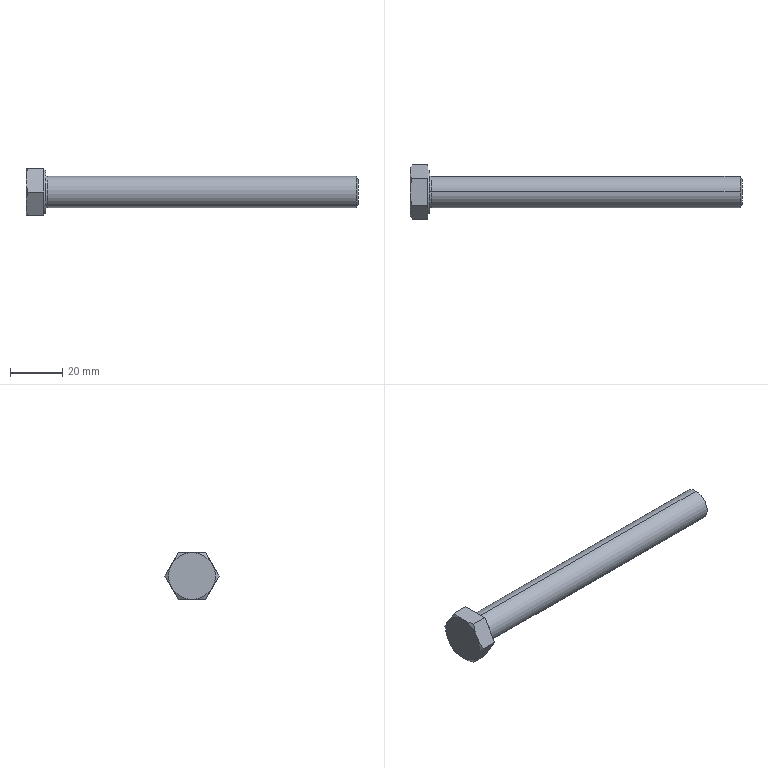Part | SolidWorks | features RevCut 3, Extrusion 1, Fillet 1, LPattern 1, Revolution 1 | 1 solid | 24 faces | box 127.5 x 20.785 x 18 mm | volume 15623 mm3 | cone 10 | plane 10 | torus 2 | cylinder 2 | commonest cylinder face diameters 12 x2
STEP:
#1=CARTESIAN_POINT('',(127.5,0.,4.701));
#2=VERTEX_POINT('',#1);
#3=CARTESIAN_POINT('',(127.5,0.,-4.701));
#4=VERTEX_POINT('',#3);
#5=CARTESIAN_POINT('',(127.5,0.,0.));
#6=DIRECTION('',(-1.,0.,0.));
#7=DIRECTION('',(0.,0.,1.));
#8=AXIS2_PLACEMENT_3D('',#5,#6,#7);
#9=CIRCLE('',#8,4.701);
#10=EDGE_CURVE('',#2,#4,#9,.T.);
#11=ORIENTED_EDGE('',*,*,#10,.T.);
#12=CARTESIAN_POINT('',(126.75,0.,-6.));
#13=VERTEX_POINT('',#12);
#14=CARTESIAN_POINT('',(126.75,0.,-6.));
#15=DIRECTION('',(-0.5,0.,-0.866));
#16=VECTOR('',#15,1000.);
#17=LINE('',#14,#16);
#18=EDGE_CURVE('',#4,#13,#17,.T.);
#19=ORIENTED_EDGE('',*,*,#18,.T.);
#20=CARTESIAN_POINT('',(126.75,0.,6.));
#21=VERTEX_POINT('',#20);
#22=CARTESIAN_POINT('',(126.75,0.,0.));
#23=DIRECTION('',(-1.,0.,0.));
#24=DIRECTION('',(0.,0.,1.));
#25=AXIS2_PLACEMENT_3D('',#22,#23,#24);
#26=CIRCLE('',#25,6.);
#27=EDGE_CURVE('',#21,#13,#26,.T.);
#28=ORIENTED_EDGE('',*,*,#27,.F.);
#29=CARTESIAN_POINT('',(126.75,0.,6.));
#30=DIRECTION('',(-0.5,0.,0.866));
#31=VECTOR('',#30,1000.);
#32=LINE('',#29,#31);
#33=EDGE_CURVE('',#2,#21,#32,.T.);
#34=ORIENTED_EDGE('',*,*,#33,.F.);
#35=EDGE_LOOP('',(#11,#19,#28,#34));
#36=FACE_OUTER_BOUND('',#35,.T.);
#37=CARTESIAN_POINT('',(126.75,0.,0.));
#38=DIRECTION('',(-1.,0.,0.));
#39=DIRECTION('',(0.,0.,1.));
#40=AXIS2_PLACEMENT_3D('',#37,#38,#39);
#41=CONICAL_SURFACE('',#40,6.,1.047);
#42=ADVANCED_FACE('',(#36),#41,.T.);
#43=CARTESIAN_POINT('',(8.1,0.,6.));
#44=VERTEX_POINT('',#43);
#45=CARTESIAN_POINT('',(8.1,0.,-6.));
#46=VERTEX_POINT('',#45);
#47=CARTESIAN_POINT('',(8.1,0.,0.));
#48=DIRECTION('',(1.,0.,0.));
#49=DIRECTION('',(0.,0.,-1.));
#50=AXIS2_PLACEMENT_3D('',#47,#48,#49);
#51=CIRCLE('',#50,6.);
#52=EDGE_CURVE('',#44,#46,#51,.T.);
#53=ORIENTED_EDGE('',*,*,#52,.F.);
#54=CARTESIAN_POINT('',(7.5,0.,6.6));
#55=VERTEX_POINT('',#54);
#56=CARTESIAN_POINT('',(8.1,0.,6.6));
#57=DIRECTION('',(0.,1.,0.));
#58=DIRECTION('',(0.,0.,1.));
#59=AXIS2_PLACEMENT_3D('',#56,#57,#58);
#60=CIRCLE('',#59,0.6);
#61=EDGE_CURVE('',#44,#55,#60,.T.);
#62=ORIENTED_EDGE('',*,*,#61,.T.);
#63=CARTESIAN_POINT('',(7.5,0.,-6.6));
#64=VERTEX_POINT('',#63);
#65=CARTESIAN_POINT('',(7.5,0.,0.));
#66=DIRECTION('',(-1.,0.,0.));
#67=DIRECTION('',(0.,0.,-1.));
#68=AXIS2_PLACEMENT_3D('',#65,#66,#67);
#69=CIRCLE('',#68,6.6);
#70=EDGE_CURVE('',#64,#55,#69,.T.);
#71=ORIENTED_EDGE('',*,*,#70,.F.);
#72=CARTESIAN_POINT('',(8.1,0.,-6.6));
#73=DIRECTION('',(0.,-1.,0.));
#74=DIRECTION('',(0.,0.,-1.));
#75=AXIS2_PLACEMENT_3D('',#72,#73,#74);
#76=CIRCLE('',#75,0.6);
#77=EDGE_CURVE('',#46,#64,#76,.T.);
#78=ORIENTED_EDGE('',*,*,#77,.F.);
#79=EDGE_LOOP('',(#53,#62,#71,#78));
#80=FACE_OUTER_BOUND('',#79,.T.);
#81=CARTESIAN_POINT('',(8.1,0.,0.));
#82=DIRECTION('',(1.,0.,0.));
#83=DIRECTION('',(0.,0.,-1.));
#84=AXIS2_PLACEMENT_3D('',#81,#82,#83);
#85=TOROIDAL_SURFACE('',#84,6.6,0.6);
#86=ADVANCED_FACE('',(#80),#85,.F.);
#87=CARTESIAN_POINT('',(7.5,0.,8.315));
#88=VERTEX_POINT('',#87);
#89=CARTESIAN_POINT('',(7.5,0.,-8.315));
#90=VERTEX_POINT('',#89);
#91=CARTESIAN_POINT('',(7.5,0.,0.));
#92=DIRECTION('',(-1.,0.,0.));
#93=DIRECTION('',(0.,0.,1.));
#94=AXIS2_PLACEMENT_3D('',#91,#92,#93);
#95=CIRCLE('',#94,8.315);
#96=EDGE_CURVE('',#88,#90,#95,.T.);
#97=ORIENTED_EDGE('',*,*,#96,.T.);
#98=CARTESIAN_POINT('',(6.9,0.,-8.661));
#99=VERTEX_POINT('',#98);
#100=CARTESIAN_POINT('',(6.9,0.,-8.661));
#101=DIRECTION('',(-0.866,0.,-0.5));
#102=VECTOR('',#101,1000.);
#103=LINE('',#100,#102);
#104=EDGE_CURVE('',#90,#99,#103,.T.);
#105=ORIENTED_EDGE('',*,*,#104,.T.);
#106=CARTESIAN_POINT('',(6.9,0.,8.661));
#107=VERTEX_POINT('',#106);
#108=CARTESIAN_POINT('',(6.9,0.,0.));
#109=DIRECTION('',(-1.,0.,0.));
#110=DIRECTION('',(0.,0.,1.));
#111=AXIS2_PLACEMENT_3D('',#108,#109,#110);
#112=CIRCLE('',#111,8.661);
#113=EDGE_CURVE('',#107,#99,#112,.T.);
#114=ORIENTED_EDGE('',*,*,#113,.F.);
#115=CARTESIAN_POINT('',(6.9,0.,8.661));
#116=DIRECTION('',(-0.866,0.,0.5));
#117=VECTOR('',#116,1000.);
#118=LINE('',#115,#117);
#119=EDGE_CURVE('',#88,#107,#118,.T.);
#120=ORIENTED_EDGE('',*,*,#119,.F.);
#121=EDGE_LOOP('',(#97,#105,#114,#120));
#122=FACE_OUTER_BOUND('',#121,.T.);
#123=CARTESIAN_POINT('',(6.9,0.,0.));
#124=DIRECTION('',(-1.,0.,0.));
#125=DIRECTION('',(0.,0.,1.));
#126=AXIS2_PLACEMENT_3D('',#123,#124,#125);
#127=CONICAL_SURFACE('',#126,8.661,0.5236);
#128=ADVANCED_FACE('',(#122),#127,.T.);
#129=ORIENTED_EDGE('',*,*,#27,.T.);
#130=CARTESIAN_POINT('',(0.,0.,-6.));
#131=DIRECTION('',(-1.,0.,0.));
#132=VECTOR('',#131,1000.);
#133=LINE('',#130,#132);
#134=EDGE_CURVE('',#13,#46,#133,.T.);
#135=ORIENTED_EDGE('',*,*,#134,.T.);
#136=CARTESIAN_POINT('',(8.1,0.,0.));
#137=DIRECTION('',(1.,0.,0.));
#138=DIRECTION('',(0.,0.,-1.));
#139=AXIS2_PLACEMENT_3D('',#136,#137,#138);
#140=CIRCLE('',#139,6.);
#141=EDGE_CURVE('',#46,#44,#140,.T.);
#142=ORIENTED_EDGE('',*,*,#141,.T.);
#143=CARTESIAN_POINT('',(0.,0.,6.));
#144=DIRECTION('',(-1.,0.,0.));
#145=VECTOR('',#144,1000.);
#146=LINE('',#143,#145);
#147=EDGE_CURVE('',#21,#44,#146,.T.);
#148=ORIENTED_EDGE('',*,*,#147,.F.);
#149=EDGE_LOOP('',(#129,#135,#142,#148));
#150=FACE_OUTER_BOUND('',#149,.T.);
#151=CARTESIAN_POINT('',(0.,0.,0.));
#152=DIRECTION('',(-1.,0.,0.));
#153=DIRECTION('',(0.,0.,1.));
#154=AXIS2_PLACEMENT_3D('',#151,#152,#153);
#155=CYLINDRICAL_SURFACE('',#154,6.);
#156=ADVANCED_FACE('',(#150),#155,.T.);
#157=ORIENTED_EDGE('',*,*,#134,.F.);
#158=CARTESIAN_POINT('',(126.75,0.,0.));
#159=DIRECTION('',(-1.,0.,0.));
#160=DIRECTION('',(0.,0.,1.));
#161=AXIS2_PLACEMENT_3D('',#158,#159,#160);
#162=CIRCLE('',#161,6.);
#163=EDGE_CURVE('',#13,#21,#162,.T.);
#164=ORIENTED_EDGE('',*,*,#163,.T.);
#165=ORIENTED_EDGE('',*,*,#147,.T.);
#166=ORIENTED_EDGE('',*,*,#52,.T.);
#167=EDGE_LOOP('',(#157,#164,#165,#166));
#168=FACE_OUTER_BOUND('',#167,.T.);
#169=CARTESIAN_POINT('',(0.,0.,0.));
#170=DIRECTION('',(-1.,0.,0.));
#171=DIRECTION('',(0.,0.,1.));
#172=AXIS2_PLACEMENT_3D('',#169,#170,#171);
#173=CYLINDRICAL_SURFACE('',#172,6.);
#174=ADVANCED_FACE('',(#168),#173,.T.);
#175=CARTESIAN_POINT('',(6.9,5.196,-9.));
#176=VERTEX_POINT('',#175);
#177=CARTESIAN_POINT('',(6.9,10.392,0.));
#178=VERTEX_POINT('',#177);
#179=CARTESIAN_POINT('',(6.9,5.196,-9.));
#180=DIRECTION('',(0.,0.5,0.866));
#181=VECTOR('',#180,1000.);
#182=LINE('',#179,#181);
#183=EDGE_CURVE('',#176,#178,#182,.T.);
#184=ORIENTED_EDGE('',*,*,#183,.F.);
#185=CARTESIAN_POINT('',(0.8038,5.196,-9.));
#186=VERTEX_POINT('',#185);
#187=CARTESIAN_POINT('',(7.5,5.196,-9.));
#188=DIRECTION('',(-1.,0.,0.));
#189=VECTOR('',#188,1000.);
#190=LINE('',#187,#189);
#191=EDGE_CURVE('',#176,#186,#190,.T.);
#192=ORIENTED_EDGE('',*,*,#191,.T.);
#193=CARTESIAN_POINT('',(0.,7.794,-4.5));
#194=VERTEX_POINT('',#193);
#195=CARTESIAN_POINT('',(0.,7.794,-4.5));
#196=CARTESIAN_POINT('',(0.,7.574,-4.882));
#197=CARTESIAN_POINT('',(0.019,7.352,-5.266));
#198=CARTESIAN_POINT('',(0.09253,6.914,-6.024));
#199=CARTESIAN_POINT('',(0.147,6.697,-6.401));
#200=CARTESIAN_POINT('',(0.357,6.048,-7.525));
#201=CARTESIAN_POINT('',(0.5591,5.62,-8.266));
#202=CARTESIAN_POINT('',(0.8038,5.196,-9.));
#203=B_SPLINE_CURVE_WITH_KNOTS('',3,(#195,#196,#197,#198,#199,#200,#201,#202),.UNSPECIFIED.,.F.,.F.,(4,2,2,4),(0.005258,0.006567,0.007877,0.0105),.UNSPECIFIED.);
#204=EDGE_CURVE('',#194,#186,#203,.T.);
#205=ORIENTED_EDGE('',*,*,#204,.F.);
#206=CARTESIAN_POINT('',(0.8038,10.392,0.));
#207=VERTEX_POINT('',#206);
#208=CARTESIAN_POINT('',(0.8038,10.392,0.));
#209=CARTESIAN_POINT('',(0.5585,9.967,-0.7361));
#210=CARTESIAN_POINT('',(0.3563,9.539,-1.478));
#211=CARTESIAN_POINT('',(0.07661,8.674,-2.976));
#212=CARTESIAN_POINT('',(0.,8.237,-3.733));
#213=CARTESIAN_POINT('',(0.,7.794,-4.5));
#214=B_SPLINE_CURVE_WITH_KNOTS('',3,(#208,#209,#210,#211,#212,#213),.UNSPECIFIED.,.F.,.F.,(4,2,4),(0.000000238,0.002629,0.005258),.UNSPECIFIED.);
#215=EDGE_CURVE('',#207,#194,#214,.T.);
#216=ORIENTED_EDGE('',*,*,#215,.F.);
#217=CARTESIAN_POINT('',(7.5,10.392,0.));
#218=DIRECTION('',(-1.,0.,0.));
#219=VECTOR('',#218,1000.);
#220=LINE('',#217,#219);
#221=EDGE_CURVE('',#178,#207,#220,.T.);
#222=ORIENTED_EDGE('',*,*,#221,.F.);
#223=EDGE_LOOP('',(#184,#192,#205,#216,#222));
#224=FACE_OUTER_BOUND('',#223,.T.);
#225=CARTESIAN_POINT('',(7.5,5.196,-9.));
#226=DIRECTION('',(0.,-0.866,0.5));
#227=DIRECTION('',(0.,-0.5,-0.866));
#228=AXIS2_PLACEMENT_3D('',#225,#226,#227);
#229=PLANE('',#228);
#230=ADVANCED_FACE('',(#224),#229,.F.);
#231=CARTESIAN_POINT('',(6.9,5.196,9.));
#232=VERTEX_POINT('',#231);
#233=CARTESIAN_POINT('',(6.9,10.392,0.));
#234=DIRECTION('',(0.,-0.5,0.866));
#235=VECTOR('',#234,1000.);
#236=LINE('',#233,#235);
#237=EDGE_CURVE('',#178,#232,#236,.T.);
#238=ORIENTED_EDGE('',*,*,#237,.F.);
#239=ORIENTED_EDGE('',*,*,#221,.T.);
#240=CARTESIAN_POINT('',(0.,7.794,4.5));
#241=VERTEX_POINT('',#240);
#242=CARTESIAN_POINT('',(0.,7.794,4.5));
#243=CARTESIAN_POINT('',(0.,8.015,4.118));
#244=CARTESIAN_POINT('',(0.019,8.236,3.734));
#245=CARTESIAN_POINT('',(0.09253,8.674,2.976));
#246=CARTESIAN_POINT('',(0.147,8.892,2.599));
#247=CARTESIAN_POINT('',(0.357,9.541,1.475));
#248=CARTESIAN_POINT('',(0.5591,9.968,0.7343));
#249=CARTESIAN_POINT('',(0.8038,10.392,0.));
#250=B_SPLINE_CURVE_WITH_KNOTS('',3,(#242,#243,#244,#245,#246,#247,#248,#249),.UNSPECIFIED.,.F.,.F.,(4,2,2,4),(0.005258,0.006567,0.007877,0.0105),.UNSPECIFIED.);
#251=EDGE_CURVE('',#241,#207,#250,.T.);
#252=ORIENTED_EDGE('',*,*,#251,.F.);
#253=CARTESIAN_POINT('',(0.8038,5.196,9.));
#254=VERTEX_POINT('',#253);
#255=CARTESIAN_POINT('',(0.8038,5.196,9.));
#256=CARTESIAN_POINT('',(0.5585,5.621,8.264));
#257=CARTESIAN_POINT('',(0.3563,6.049,7.522));
#258=CARTESIAN_POINT('',(0.07661,6.914,6.024));
#259=CARTESIAN_POINT('',(0.,7.352,5.267));
#260=CARTESIAN_POINT('',(0.,7.794,4.5));
#261=B_SPLINE_CURVE_WITH_KNOTS('',3,(#255,#256,#257,#258,#259,#260),.UNSPECIFIED.,.F.,.F.,(4,2,4),(0.000000238,0.002629,0.005258),.UNSPECIFIED.);
#262=EDGE_CURVE('',#254,#241,#261,.T.);
#263=ORIENTED_EDGE('',*,*,#262,.F.);
#264=CARTESIAN_POINT('',(7.5,5.196,9.));
#265=DIRECTION('',(-1.,0.,0.));
#266=VECTOR('',#265,1000.);
#267=LINE('',#264,#266);
#268=EDGE_CURVE('',#232,#254,#267,.T.);
#269=ORIENTED_EDGE('',*,*,#268,.F.);
#270=EDGE_LOOP('',(#238,#239,#252,#263,#269));
#271=FACE_OUTER_BOUND('',#270,.T.);
#272=CARTESIAN_POINT('',(7.5,10.392,0.));
#273=DIRECTION('',(0.,-0.866,-0.5));
#274=DIRECTION('',(0.,0.5,-0.866));
#275=AXIS2_PLACEMENT_3D('',#272,#273,#274);
#276=PLANE('',#275);
#277=ADVANCED_FACE('',(#271),#276,.F.);
#278=CARTESIAN_POINT('',(6.9,-5.196,9.));
#279=VERTEX_POINT('',#278);
#280=CARTESIAN_POINT('',(6.9,5.196,9.));
#281=DIRECTION('',(0.,-1.,0.));
#282=VECTOR('',#281,1000.);
#283=LINE('',#280,#282);
#284=EDGE_CURVE('',#232,#279,#283,.T.);
#285=ORIENTED_EDGE('',*,*,#284,.F.);
#286=ORIENTED_EDGE('',*,*,#268,.T.);
#287=CARTESIAN_POINT('',(0.,0.,9.));
#288=VERTEX_POINT('',#287);
#289=CARTESIAN_POINT('',(0.,0.,9.));
#290=CARTESIAN_POINT('',(0.,0.4401,9.));
#291=CARTESIAN_POINT('',(0.01885,0.8832,9.));
#292=CARTESIAN_POINT('',(0.09319,1.767,9.));
#293=CARTESIAN_POINT('',(0.1482,2.204,9.));
#294=CARTESIAN_POINT('',(0.3593,3.505,9.));
#295=CARTESIAN_POINT('',(0.5612,4.356,9.));
#296=CARTESIAN_POINT('',(0.8038,5.196,9.));
#297=B_SPLINE_CURVE_WITH_KNOTS('',3,(#289,#290,#291,#292,#293,#294,#295,#296),.UNSPECIFIED.,.F.,.F.,(4,2,2,4),(0.01498,0.0163,0.01761,0.02025),.UNSPECIFIED.);
#298=EDGE_CURVE('',#288,#254,#297,.T.);
#299=ORIENTED_EDGE('',*,*,#298,.F.);
#300=CARTESIAN_POINT('',(0.8038,-5.196,9.));
#301=VERTEX_POINT('',#300);
#302=CARTESIAN_POINT('',(0.8038,-5.196,9.));
#303=CARTESIAN_POINT('',(0.5595,-4.35,9.));
#304=CARTESIAN_POINT('',(0.3552,-3.485,9.));
#305=CARTESIAN_POINT('',(0.07569,-1.752,9.));
#306=CARTESIAN_POINT('',(0.,-0.8794,9.));
#307=CARTESIAN_POINT('',(0.,0.,9.));
#308=B_SPLINE_CURVE_WITH_KNOTS('',3,(#302,#303,#304,#305,#306,#307),.UNSPECIFIED.,.F.,.F.,(4,2,4),(0.00972,0.01235,0.01498),.UNSPECIFIED.);
#309=EDGE_CURVE('',#301,#288,#308,.T.);
#310=ORIENTED_EDGE('',*,*,#309,.F.);
#311=CARTESIAN_POINT('',(7.5,-5.196,9.));
#312=DIRECTION('',(-1.,0.,0.));
#313=VECTOR('',#312,1000.);
#314=LINE('',#311,#313);
#315=EDGE_CURVE('',#279,#301,#314,.T.);
#316=ORIENTED_EDGE('',*,*,#315,.F.);
#317=EDGE_LOOP('',(#285,#286,#299,#310,#316));
#318=FACE_OUTER_BOUND('',#317,.T.);
#319=CARTESIAN_POINT('',(7.5,5.196,9.));
#320=DIRECTION('',(0.,0.,-1.));
#321=DIRECTION('',(-1.,0.,0.));
#322=AXIS2_PLACEMENT_3D('',#319,#320,#321);
#323=PLANE('',#322);
#324=ADVANCED_FACE('',(#318),#323,.F.);
#325=CARTESIAN_POINT('',(6.9,-10.392,0.));
#326=VERTEX_POINT('',#325);
#327=CARTESIAN_POINT('',(6.9,-10.392,0.));
#328=DIRECTION('',(0.,-0.5,-0.866));
#329=VECTOR('',#328,1000.);
#330=LINE('',#327,#329);
#331=EDGE_CURVE('',#279,#326,#330,.T.);
#332=ORIENTED_EDGE('',*,*,#331,.F.);
#333=ORIENTED_EDGE('',*,*,#315,.T.);
#334=CARTESIAN_POINT('',(0.,-7.794,4.5));
#335=VERTEX_POINT('',#334);
#336=CARTESIAN_POINT('',(0.,-7.794,4.5));
#337=CARTESIAN_POINT('',(0.,-7.574,4.882));
#338=CARTESIAN_POINT('',(0.019,-7.352,5.266));
#339=CARTESIAN_POINT('',(0.09253,-6.914,6.024));
#340=CARTESIAN_POINT('',(0.147,-6.697,6.401));
#341=CARTESIAN_POINT('',(0.357,-6.048,7.525));
#342=CARTESIAN_POINT('',(0.5591,-5.62,8.266));
#343=CARTESIAN_POINT('',(0.8038,-5.196,9.));
#344=B_SPLINE_CURVE_WITH_KNOTS('',3,(#336,#337,#338,#339,#340,#341,#342,#343),.UNSPECIFIED.,.F.,.F.,(4,2,2,4),(0.005258,0.006567,0.007877,0.0105),.UNSPECIFIED.);
#345=EDGE_CURVE('',#335,#301,#344,.T.);
#346=ORIENTED_EDGE('',*,*,#345,.F.);
#347=CARTESIAN_POINT('',(0.8038,-10.392,0.));
#348=VERTEX_POINT('',#347);
#349=CARTESIAN_POINT('',(0.8038,-10.392,0.));
#350=CARTESIAN_POINT('',(0.5585,-9.967,0.7361));
#351=CARTESIAN_POINT('',(0.3563,-9.539,1.478));
#352=CARTESIAN_POINT('',(0.07661,-8.674,2.976));
#353=CARTESIAN_POINT('',(0.,-8.237,3.733));
#354=CARTESIAN_POINT('',(0.,-7.794,4.5));
#355=B_SPLINE_CURVE_WITH_KNOTS('',3,(#349,#350,#351,#352,#353,#354),.UNSPECIFIED.,.F.,.F.,(4,2,4),(0.000000238,0.002629,0.005258),.UNSPECIFIED.);
#356=EDGE_CURVE('',#348,#335,#355,.T.);
#357=ORIENTED_EDGE('',*,*,#356,.F.);
#358=CARTESIAN_POINT('',(7.5,-10.392,0.));
#359=DIRECTION('',(-1.,0.,0.));
#360=VECTOR('',#359,1000.);
#361=LINE('',#358,#360);
#362=EDGE_CURVE('',#326,#348,#361,.T.);
#363=ORIENTED_EDGE('',*,*,#362,.F.);
#364=EDGE_LOOP('',(#332,#333,#346,#357,#363));
#365=FACE_OUTER_BOUND('',#364,.T.);
#366=CARTESIAN_POINT('',(7.5,-10.392,0.));
#367=DIRECTION('',(0.,0.866,-0.5));
#368=DIRECTION('',(0.,0.5,0.866));
#369=AXIS2_PLACEMENT_3D('',#366,#367,#368);
#370=PLANE('',#369);
#371=ADVANCED_FACE('',(#365),#370,.F.);
#372=CARTESIAN_POINT('',(6.9,-5.196,-9.));
#373=VERTEX_POINT('',#372);
#374=CARTESIAN_POINT('',(6.9,-5.196,-9.));
#375=DIRECTION('',(0.,0.5,-0.866));
#376=VECTOR('',#375,1000.);
#377=LINE('',#374,#376);
#378=EDGE_CURVE('',#326,#373,#377,.T.);
#379=ORIENTED_EDGE('',*,*,#378,.F.);
#380=ORIENTED_EDGE('',*,*,#362,.T.);
#381=CARTESIAN_POINT('',(0.,-7.794,-4.5));
#382=VERTEX_POINT('',#381);
#383=CARTESIAN_POINT('',(0.,-7.794,-4.5));
#384=CARTESIAN_POINT('',(0.,-8.015,-4.118));
#385=CARTESIAN_POINT('',(0.019,-8.236,-3.734));
#386=CARTESIAN_POINT('',(0.09253,-8.674,-2.976));
#387=CARTESIAN_POINT('',(0.147,-8.892,-2.599));
#388=CARTESIAN_POINT('',(0.357,-9.541,-1.475));
#389=CARTESIAN_POINT('',(0.5591,-9.968,-0.7343));
#390=CARTESIAN_POINT('',(0.8038,-10.392,0.));
#391=B_SPLINE_CURVE_WITH_KNOTS('',3,(#383,#384,#385,#386,#387,#388,#389,#390),.UNSPECIFIED.,.F.,.F.,(4,2,2,4),(0.005258,0.006567,0.007877,0.0105),.UNSPECIFIED.);
#392=EDGE_CURVE('',#382,#348,#391,.T.);
#393=ORIENTED_EDGE('',*,*,#392,.F.);
#394=CARTESIAN_POINT('',(0.8038,-5.196,-9.));
#395=VERTEX_POINT('',#394);
#396=CARTESIAN_POINT('',(0.8038,-5.196,-9.));
#397=CARTESIAN_POINT('',(0.5585,-5.621,-8.264));
#398=CARTESIAN_POINT('',(0.3563,-6.049,-7.522));
#399=CARTESIAN_POINT('',(0.07661,-6.914,-6.024));
#400=CARTESIAN_POINT('',(0.,-7.352,-5.267));
#401=CARTESIAN_POINT('',(0.,-7.794,-4.5));
#402=B_SPLINE_CURVE_WITH_KNOTS('',3,(#396,#397,#398,#399,#400,#401),.UNSPECIFIED.,.F.,.F.,(4,2,4),(0.000000238,0.002629,0.005258),.UNSPECIFIED.);
#403=EDGE_CURVE('',#395,#382,#402,.T.);
#404=ORIENTED_EDGE('',*,*,#403,.F.);
#405=CARTESIAN_POINT('',(7.5,-5.196,-9.));
#406=DIRECTION('',(-1.,0.,0.));
#407=VECTOR('',#406,1000.);
#408=LINE('',#405,#407);
#409=EDGE_CURVE('',#373,#395,#408,.T.);
#410=ORIENTED_EDGE('',*,*,#409,.F.);
#411=EDGE_LOOP('',(#379,#380,#393,#404,#410));
#412=FACE_OUTER_BOUND('',#411,.T.);
#413=CARTESIAN_POINT('',(7.5,-5.196,-9.));
#414=DIRECTION('',(0.,0.866,0.5));
#415=DIRECTION('',(0.,-0.5,0.866));
#416=AXIS2_PLACEMENT_3D('',#413,#414,#415);
#417=PLANE('',#416);
#418=ADVANCED_FACE('',(#412),#417,.F.);
#419=CARTESIAN_POINT('',(6.9,5.196,-9.));
#420=DIRECTION('',(0.,1.,0.));
#421=VECTOR('',#420,1000.);
#422=LINE('',#419,#421);
#423=EDGE_CURVE('',#373,#176,#422,.T.);
#424=ORIENTED_EDGE('',*,*,#423,.F.);
#425=ORIENTED_EDGE('',*,*,#409,.T.);
#426=CARTESIAN_POINT('',(0.,0.,-9.));
#427=VERTEX_POINT('',#426);
#428=CARTESIAN_POINT('',(0.,0.,-9.));
#429=CARTESIAN_POINT('',(0.,-0.8794,-9.));
#430=CARTESIAN_POINT('',(0.07569,-1.752,-9.));
#431=CARTESIAN_POINT('',(0.3552,-3.485,-9.));
#432=CARTESIAN_POINT('',(0.5595,-4.35,-9.));
#433=CARTESIAN_POINT('',(0.8038,-5.196,-9.));
#434=B_SPLINE_CURVE_WITH_KNOTS('',3,(#428,#429,#430,#431,#432,#433),.UNSPECIFIED.,.F.,.F.,(4,2,4),(0.03045,0.03308,0.03571),.UNSPECIFIED.);
#435=EDGE_CURVE('',#427,#395,#434,.T.);
#436=ORIENTED_EDGE('',*,*,#435,.F.);
#437=CARTESIAN_POINT('',(0.8038,5.196,-9.));
#438=CARTESIAN_POINT('',(0.5612,4.356,-9.));
#439=CARTESIAN_POINT('',(0.3593,3.505,-9.));
#440=CARTESIAN_POINT('',(0.1482,2.204,-9.));
#441=CARTESIAN_POINT('',(0.09319,1.767,-9.));
#442=CARTESIAN_POINT('',(0.01885,0.8832,-9.));
#443=CARTESIAN_POINT('',(0.,0.4401,-9.));
#444=CARTESIAN_POINT('',(0.,0.,-9.));
#445=B_SPLINE_CURVE_WITH_KNOTS('',3,(#437,#438,#439,#440,#441,#442,#443,#444),.UNSPECIFIED.,.F.,.F.,(4,2,2,4),(0.02519,0.02782,0.02914,0.03045),.UNSPECIFIED.);
#446=EDGE_CURVE('',#186,#427,#445,.T.);
#447=ORIENTED_EDGE('',*,*,#446,.F.);
#448=ORIENTED_EDGE('',*,*,#191,.F.);
#449=EDGE_LOOP('',(#424,#425,#436,#447,#448));
#450=FACE_OUTER_BOUND('',#449,.T.);
#451=CARTESIAN_POINT('',(7.5,5.196,-9.));
#452=DIRECTION('',(0.,0.,1.));
#453=DIRECTION('',(0.,-1.,0.));
#454=AXIS2_PLACEMENT_3D('',#451,#452,#453);
#455=PLANE('',#454);
#456=ADVANCED_FACE('',(#450),#455,.F.);
#457=ORIENTED_EDGE('',*,*,#403,.T.);
#458=CARTESIAN_POINT('',(0.,0.,0.));
#459=DIRECTION('',(1.,0.,0.));
#460=DIRECTION('',(0.,0.,-1.));
#461=AXIS2_PLACEMENT_3D('',#458,#459,#460);
#462=CIRCLE('',#461,9.);
#463=EDGE_CURVE('',#382,#427,#462,.T.);
#464=ORIENTED_EDGE('',*,*,#463,.T.);
#465=ORIENTED_EDGE('',*,*,#435,.T.);
#466=EDGE_LOOP('',(#457,#464,#465));
#467=FACE_OUTER_BOUND('',#466,.T.);
#468=CARTESIAN_POINT('',(0.,0.,0.));
#469=DIRECTION('',(1.,0.,0.));
#470=DIRECTION('',(0.,0.,-1.));
#471=AXIS2_PLACEMENT_3D('',#468,#469,#470);
#472=CONICAL_SURFACE('',#471,9.,1.047);
#473=ADVANCED_FACE('',(#467),#472,.T.);
#474=ORIENTED_EDGE('',*,*,#356,.T.);
#475=CARTESIAN_POINT('',(0.,0.,0.));
#476=DIRECTION('',(1.,0.,0.));
#477=DIRECTION('',(0.,0.,-1.));
#478=AXIS2_PLACEMENT_3D('',#475,#476,#477);
#479=CIRCLE('',#478,9.);
#480=EDGE_CURVE('',#335,#382,#479,.T.);
#481=ORIENTED_EDGE('',*,*,#480,.T.);
#482=ORIENTED_EDGE('',*,*,#392,.T.);
#483=EDGE_LOOP('',(#474,#481,#482));
#484=FACE_OUTER_BOUND('',#483,.T.);
#485=CARTESIAN_POINT('',(0.,0.,0.));
#486=DIRECTION('',(1.,0.,0.));
#487=DIRECTION('',(0.,0.,-1.));
#488=AXIS2_PLACEMENT_3D('',#485,#486,#487);
#489=CONICAL_SURFACE('',#488,9.,1.047);
#490=ADVANCED_FACE('',(#484),#489,.T.);
#491=ORIENTED_EDGE('',*,*,#309,.T.);
#492=CARTESIAN_POINT('',(0.,0.,0.));
#493=DIRECTION('',(1.,0.,0.));
#494=DIRECTION('',(0.,0.,-1.));
#495=AXIS2_PLACEMENT_3D('',#492,#493,#494);
#496=CIRCLE('',#495,9.);
#497=EDGE_CURVE('',#288,#335,#496,.T.);
#498=ORIENTED_EDGE('',*,*,#497,.T.);
#499=ORIENTED_EDGE('',*,*,#345,.T.);
#500=EDGE_LOOP('',(#491,#498,#499));
#501=FACE_OUTER_BOUND('',#500,.T.);
#502=CARTESIAN_POINT('',(0.,0.,0.));
#503=DIRECTION('',(1.,0.,0.));
#504=DIRECTION('',(0.,0.,-1.));
#505=AXIS2_PLACEMENT_3D('',#502,#503,#504);
#506=CONICAL_SURFACE('',#505,9.,1.047);
#507=ADVANCED_FACE('',(#501),#506,.T.);
#508=ORIENTED_EDGE('',*,*,#298,.T.);
#509=ORIENTED_EDGE('',*,*,#262,.T.);
#510=CARTESIAN_POINT('',(0.,0.,0.));
#511=DIRECTION('',(-1.,0.,0.));
#512=DIRECTION('',(0.,0.,1.));
#513=AXIS2_PLACEMENT_3D('',#510,#511,#512);
#514=CIRCLE('',#513,9.);
#515=EDGE_CURVE('',#288,#241,#514,.T.);
#516=ORIENTED_EDGE('',*,*,#515,.F.);
#517=EDGE_LOOP('',(#508,#509,#516));
#518=FACE_OUTER_BOUND('',#517,.T.);
#519=CARTESIAN_POINT('',(0.,0.,0.));
#520=DIRECTION('',(1.,0.,0.));
#521=DIRECTION('',(0.,0.,-1.));
#522=AXIS2_PLACEMENT_3D('',#519,#520,#521);
#523=CONICAL_SURFACE('',#522,9.,1.047);
#524=ADVANCED_FACE('',(#518),#523,.T.);
#525=ORIENTED_EDGE('',*,*,#251,.T.);
#526=ORIENTED_EDGE('',*,*,#215,.T.);
#527=CARTESIAN_POINT('',(0.,0.,0.));
#528=DIRECTION('',(1.,0.,0.));
#529=DIRECTION('',(0.,0.,-1.));
#530=AXIS2_PLACEMENT_3D('',#527,#528,#529);
#531=CIRCLE('',#530,9.);
#532=EDGE_CURVE('',#194,#241,#531,.T.);
#533=ORIENTED_EDGE('',*,*,#532,.T.);
#534=EDGE_LOOP('',(#525,#526,#533));
#535=FACE_OUTER_BOUND('',#534,.T.);
#536=CARTESIAN_POINT('',(0.,0.,0.));
#537=DIRECTION('',(1.,0.,0.));
#538=DIRECTION('',(0.,0.,-1.));
#539=AXIS2_PLACEMENT_3D('',#536,#537,#538);
#540=CONICAL_SURFACE('',#539,9.,1.047);
#541=ADVANCED_FACE('',(#535),#540,.T.);
#542=ORIENTED_EDGE('',*,*,#204,.T.);
#543=ORIENTED_EDGE('',*,*,#446,.T.);
#544=CARTESIAN_POINT('',(0.,0.,0.));
#545=DIRECTION('',(1.,0.,0.));
#546=DIRECTION('',(0.,0.,-1.));
#547=AXIS2_PLACEMENT_3D('',#544,#545,#546);
#548=CIRCLE('',#547,9.);
#549=EDGE_CURVE('',#427,#194,#548,.T.);
#550=ORIENTED_EDGE('',*,*,#549,.T.);
#551=EDGE_LOOP('',(#542,#543,#550));
#552=FACE_OUTER_BOUND('',#551,.T.);
#553=CARTESIAN_POINT('',(0.,0.,0.));
#554=DIRECTION('',(1.,0.,0.));
#555=DIRECTION('',(0.,0.,-1.));
#556=AXIS2_PLACEMENT_3D('',#553,#554,#555);
#557=CONICAL_SURFACE('',#556,9.,1.047);
#558=ADVANCED_FACE('',(#552),#557,.T.);
#559=ORIENTED_EDGE('',*,*,#549,.F.);
#560=ORIENTED_EDGE('',*,*,#463,.F.);
#561=ORIENTED_EDGE('',*,*,#480,.F.);
#562=ORIENTED_EDGE('',*,*,#497,.F.);
#563=ORIENTED_EDGE('',*,*,#515,.T.);
#564=ORIENTED_EDGE('',*,*,#532,.F.);
#565=EDGE_LOOP('',(#559,#560,#561,#562,#563,#564));
#566=FACE_OUTER_BOUND('',#565,.T.);
#567=CARTESIAN_POINT('',(0.,0.,-18.));
#568=DIRECTION('',(1.,0.,0.));
#569=DIRECTION('',(0.,0.,-1.));
#570=AXIS2_PLACEMENT_3D('',#567,#568,#569);
#571=PLANE('',#570);
#572=ADVANCED_FACE('',(#566),#571,.F.);
#573=ORIENTED_EDGE('',*,*,#113,.T.);
#574=CARTESIAN_POINT('',(6.9,0.,0.));
#575=DIRECTION('',(-1.,0.,0.));
#576=DIRECTION('',(0.,0.,1.));
#577=AXIS2_PLACEMENT_3D('',#574,#575,#576);
#578=CIRCLE('',#577,8.661);
#579=EDGE_CURVE('',#99,#107,#578,.T.);
#580=ORIENTED_EDGE('',*,*,#579,.T.);
#581=EDGE_LOOP('',(#573,#580));
#582=FACE_BOUND('',#581,.T.);
#583=ORIENTED_EDGE('',*,*,#183,.T.);
#584=ORIENTED_EDGE('',*,*,#237,.T.);
#585=ORIENTED_EDGE('',*,*,#284,.T.);
#586=ORIENTED_EDGE('',*,*,#331,.T.);
#587=ORIENTED_EDGE('',*,*,#378,.T.);
#588=ORIENTED_EDGE('',*,*,#423,.T.);
#589=EDGE_LOOP('',(#583,#584,#585,#586,#587,#588));
#590=FACE_OUTER_BOUND('',#589,.T.);
#591=CARTESIAN_POINT('',(6.9,8.661,0.));
#592=DIRECTION('',(1.,0.,0.));
#593=DIRECTION('',(0.,0.,-1.));
#594=AXIS2_PLACEMENT_3D('',#591,#592,#593);
#595=PLANE('',#594);
#596=ADVANCED_FACE('',(#582,#590),#595,.T.);
#597=ORIENTED_EDGE('',*,*,#104,.F.);
#598=CARTESIAN_POINT('',(7.5,0.,0.));
#599=DIRECTION('',(-1.,0.,0.));
#600=DIRECTION('',(0.,0.,1.));
#601=AXIS2_PLACEMENT_3D('',#598,#599,#600);
#602=CIRCLE('',#601,8.315);
#603=EDGE_CURVE('',#90,#88,#602,.T.);
#604=ORIENTED_EDGE('',*,*,#603,.T.);
#605=ORIENTED_EDGE('',*,*,#119,.T.);
#606=ORIENTED_EDGE('',*,*,#579,.F.);
#607=EDGE_LOOP('',(#597,#604,#605,#606));
#608=FACE_OUTER_BOUND('',#607,.T.);
#609=CARTESIAN_POINT('',(6.9,0.,0.));
#610=DIRECTION('',(-1.,0.,0.));
#611=DIRECTION('',(0.,0.,1.));
#612=AXIS2_PLACEMENT_3D('',#609,#610,#611);
#613=CONICAL_SURFACE('',#612,8.661,0.5236);
#614=ADVANCED_FACE('',(#608),#613,.T.);
#615=ORIENTED_EDGE('',*,*,#70,.T.);
#616=CARTESIAN_POINT('',(7.5,0.,0.));
#617=DIRECTION('',(-1.,0.,0.));
#618=DIRECTION('',(0.,0.,-1.));
#619=AXIS2_PLACEMENT_3D('',#616,#617,#618);
#620=CIRCLE('',#619,6.6);
#621=EDGE_CURVE('',#55,#64,#620,.T.);
#622=ORIENTED_EDGE('',*,*,#621,.T.);
#623=EDGE_LOOP('',(#615,#622));
#624=FACE_BOUND('',#623,.T.);
#625=ORIENTED_EDGE('',*,*,#96,.F.);
#626=ORIENTED_EDGE('',*,*,#603,.F.);
#627=EDGE_LOOP('',(#625,#626));
#628=FACE_OUTER_BOUND('',#627,.T.);
#629=CARTESIAN_POINT('',(7.5,0.,-18.));
#630=DIRECTION('',(1.,0.,0.));
#631=DIRECTION('',(0.,0.,-1.));
#632=AXIS2_PLACEMENT_3D('',#629,#630,#631);
#633=PLANE('',#632);
#634=ADVANCED_FACE('',(#624,#628),#633,.T.);
#635=ORIENTED_EDGE('',*,*,#61,.F.);
#636=ORIENTED_EDGE('',*,*,#141,.F.);
#637=ORIENTED_EDGE('',*,*,#77,.T.);
#638=ORIENTED_EDGE('',*,*,#621,.F.);
#639=EDGE_LOOP('',(#635,#636,#637,#638));
#640=FACE_OUTER_BOUND('',#639,.T.);
#641=CARTESIAN_POINT('',(8.1,0.,0.));
#642=DIRECTION('',(1.,0.,0.));
#643=DIRECTION('',(0.,0.,-1.));
#644=AXIS2_PLACEMENT_3D('',#641,#642,#643);
#645=TOROIDAL_SURFACE('',#644,6.6,0.6);
#646=ADVANCED_FACE('',(#640),#645,.F.);
#647=ORIENTED_EDGE('',*,*,#18,.F.);
#648=CARTESIAN_POINT('',(127.5,0.,0.));
#649=DIRECTION('',(-1.,0.,0.));
#650=DIRECTION('',(0.,0.,1.));
#651=AXIS2_PLACEMENT_3D('',#648,#649,#650);
#652=CIRCLE('',#651,4.701);
#653=EDGE_CURVE('',#4,#2,#652,.T.);
#654=ORIENTED_EDGE('',*,*,#653,.T.);
#655=ORIENTED_EDGE('',*,*,#33,.T.);
#656=ORIENTED_EDGE('',*,*,#163,.F.);
#657=EDGE_LOOP('',(#647,#654,#655,#656));
#658=FACE_OUTER_BOUND('',#657,.T.);
#659=CARTESIAN_POINT('',(126.75,0.,0.));
#660=DIRECTION('',(-1.,0.,0.));
#661=DIRECTION('',(0.,0.,1.));
#662=AXIS2_PLACEMENT_3D('',#659,#660,#661);
#663=CONICAL_SURFACE('',#662,6.,1.047);
#664=ADVANCED_FACE('',(#658),#663,.T.);
#665=ORIENTED_EDGE('',*,*,#10,.F.);
#666=ORIENTED_EDGE('',*,*,#653,.F.);
#667=EDGE_LOOP('',(#665,#666));
#668=FACE_OUTER_BOUND('',#667,.T.);
#669=CARTESIAN_POINT('',(127.5,0.,0.));
#670=DIRECTION('',(-1.,0.,0.));
#671=DIRECTION('',(0.,0.,1.));
#672=AXIS2_PLACEMENT_3D('',#669,#670,#671);
#673=PLANE('',#672);
#674=ADVANCED_FACE('',(#668),#673,.F.);
#675=CLOSED_SHELL('',(#42,#86,#128,#156,#174,#230,#277,#324,#371,#418,#456,#473,#490,#507,#524,#541,#558,#572,#596,#614,#634,#646,#664,#674));
#676=MANIFOLD_SOLID_BREP('',#675);
#677=CARTESIAN_POINT('',(0.,0.,0.));
#678=DIRECTION('',(0.,0.,1.));
#679=DIRECTION('',(1.,0.,0.));
#680=AXIS2_PLACEMENT_3D('',#677,#678,#679);
#681=(LENGTH_UNIT()NAMED_UNIT(*)SI_UNIT(.MILLI.,.METRE.));
#682=UNCERTAINTY_MEASURE_WITH_UNIT(LENGTH_MEASURE(0.00001),#681,'','');
#683=(NAMED_UNIT(*)PLANE_ANGLE_UNIT()SI_UNIT($,.RADIAN.));
#684=(NAMED_UNIT(*)SI_UNIT($,.STERADIAN.)SOLID_ANGLE_UNIT());
#685=(GEOMETRIC_REPRESENTATION_CONTEXT(3)GLOBAL_UNCERTAINTY_ASSIGNED_CONTEXT((#682))GLOBAL_UNIT_ASSIGNED_CONTEXT((#681,#683,#684))REPRESENTATION_CONTEXT('',''));
#686=ADVANCED_BREP_SHAPE_REPRESENTATION('',(#676,#680),#685);